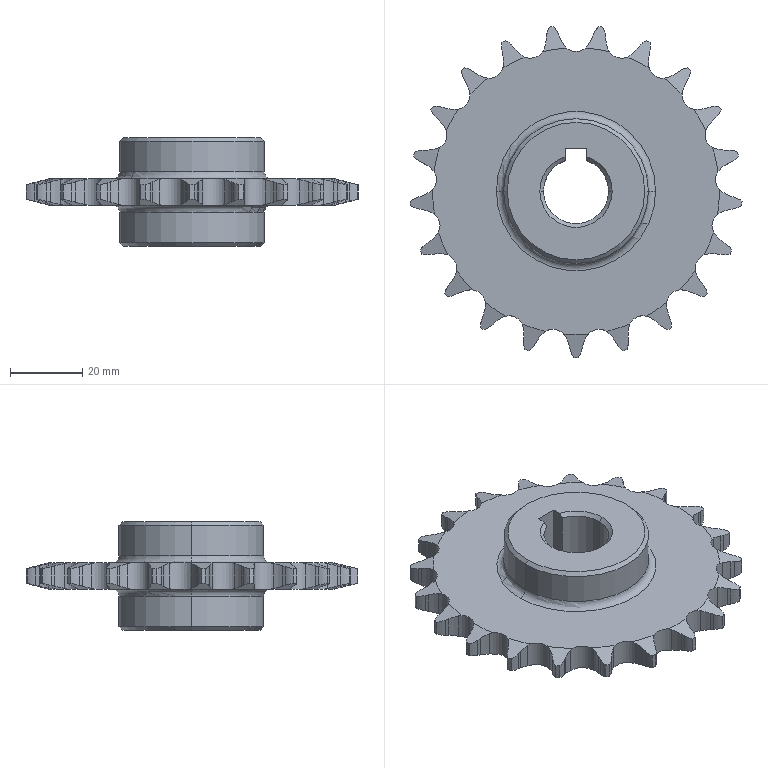Part | STEP file | 06-Small sprocket 4 | 1 solid | 240 faces | box 91.703 x 91.451 x 30 mm | volume 58578 mm3 | cylinder 133 | cone 54 | plane 49 | torus 4 | commonest cylinder face diameters 13.116 x42 20.647 x42 7.967 x21 91.879 x21 40 x4 18 x3